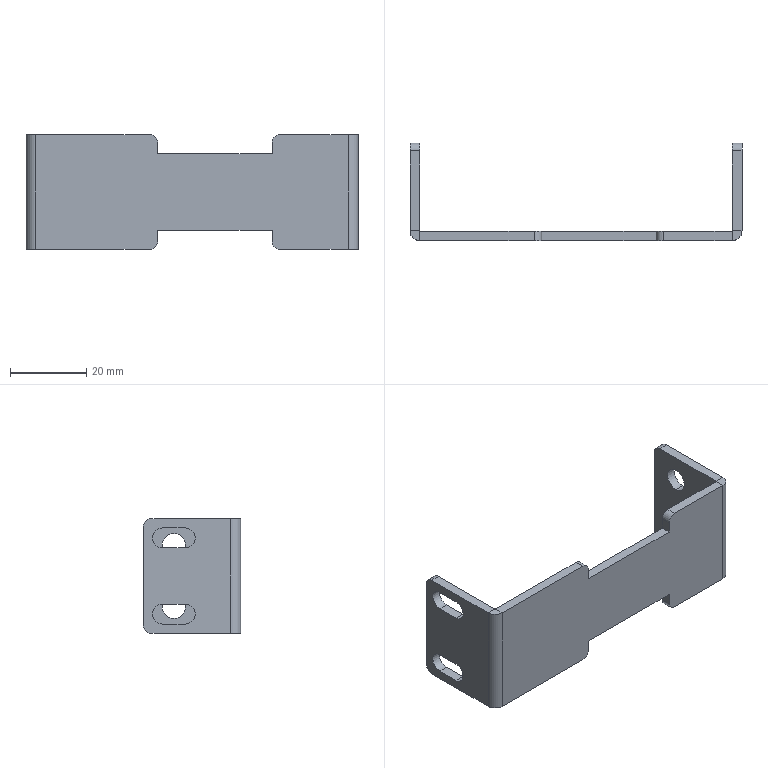Part | STEP file | 1 solid | 50 faces | box 87 x 25.5 x 30 mm | volume 8708 mm3 | plane 30 | cylinder 20 | commonest cylinder face diameters 4 x8 5.2 x6 6.2 x4 0.2 x2